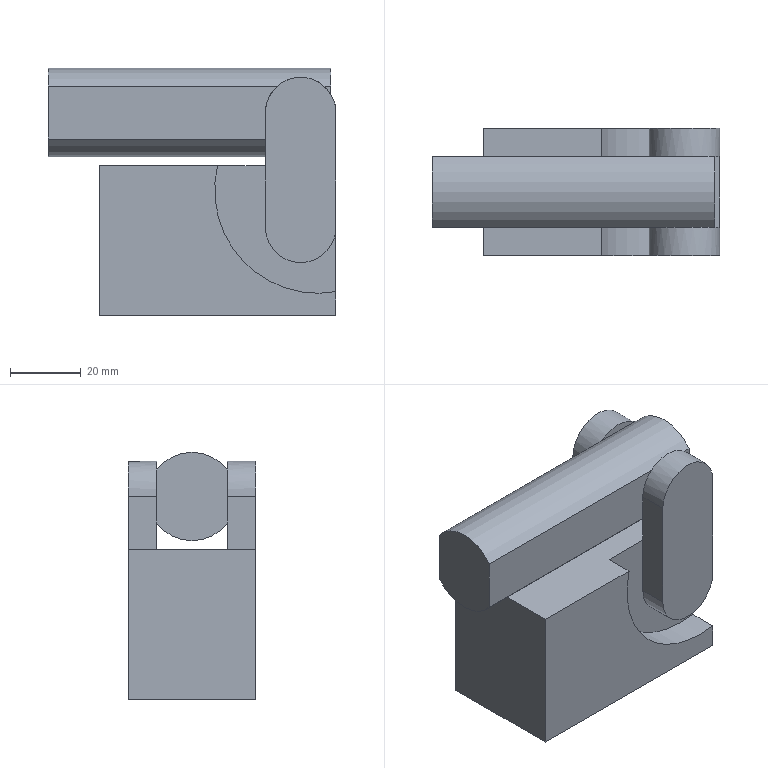Part | STEP file | Positioning_id1910_x_t | 1 solid | 30 faces | box 81.5 x 36 x 70 mm | volume 136244 mm3 | plane 22 | cylinder 8 | commonest cylinder face diameters 20 x4 25 x2 58.558 x2